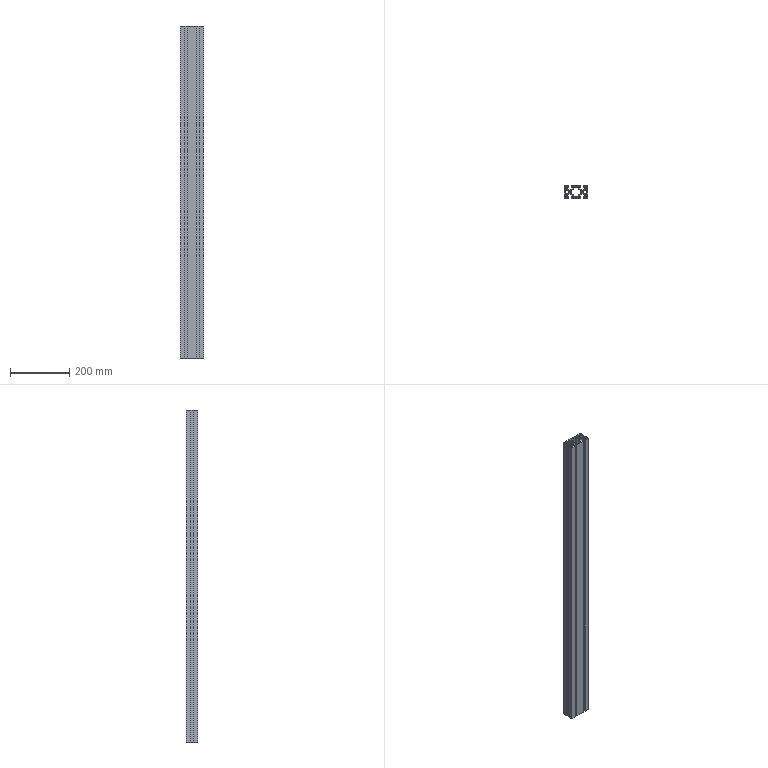Part | NX | 1 solid | 88 faces | box 80 x 40 x 1120 mm | volume 1356854 mm3 | plane 78 | cylinder 10 | commonest cylinder face diameters 6 x4 8 x4 6.75 x2